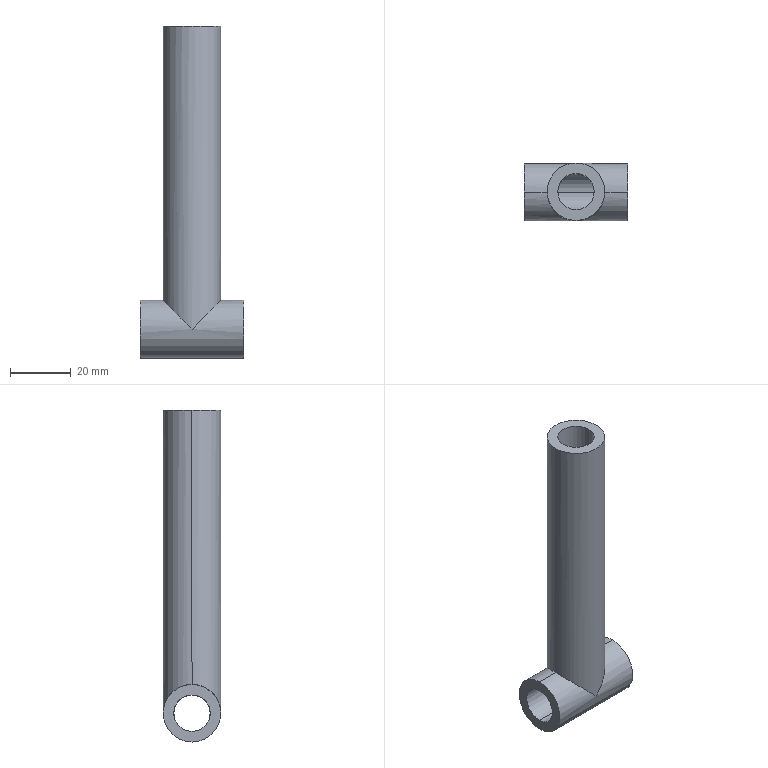Part | NX | features BREP 1 | 1 solid | 11 faces | box 34 x 19 x 109.5 mm | volume 21127 mm3 | cylinder 8 | plane 3 | commonest cylinder face diameters 12 x4 19 x4
STEP:
#1=CARTESIAN_POINT('',(34.,0.,6.));
#2=VERTEX_POINT('',#1);
#3=CARTESIAN_POINT('',(34.,0.,-6.));
#4=VERTEX_POINT('',#3);
#5=CARTESIAN_POINT('',(34.,0.,0.));
#6=DIRECTION('',(1.,0.,0.));
#7=DIRECTION('',(0.,0.,-1.));
#8=AXIS2_PLACEMENT_3D('',#5,#6,#7);
#9=CIRCLE('',#8,6.);
#10=EDGE_CURVE('',#2,#4,#9,.T.);
#11=ORIENTED_EDGE('',*,*,#10,.T.);
#12=CARTESIAN_POINT('',(0.,0.,-6.));
#13=VERTEX_POINT('',#12);
#14=CARTESIAN_POINT('',(34.001,0.,-6.));
#15=DIRECTION('',(-1.,0.,0.));
#16=VECTOR('',#15,1000.);
#17=LINE('',#14,#16);
#18=EDGE_CURVE('',#4,#13,#17,.T.);
#19=ORIENTED_EDGE('',*,*,#18,.T.);
#20=CARTESIAN_POINT('',(0.,0.,6.));
#21=VERTEX_POINT('',#20);
#22=CARTESIAN_POINT('',(0.,0.,0.));
#23=DIRECTION('',(1.,0.,0.));
#24=DIRECTION('',(0.,0.,-1.));
#25=AXIS2_PLACEMENT_3D('',#22,#23,#24);
#26=CIRCLE('',#25,6.);
#27=EDGE_CURVE('',#21,#13,#26,.T.);
#28=ORIENTED_EDGE('',*,*,#27,.F.);
#29=CARTESIAN_POINT('',(11.,0.,6.));
#30=VERTEX_POINT('',#29);
#31=CARTESIAN_POINT('',(34.001,0.,6.));
#32=DIRECTION('',(-1.,0.,0.));
#33=VECTOR('',#32,1000.);
#34=LINE('',#31,#33);
#35=EDGE_CURVE('',#30,#21,#34,.T.);
#36=ORIENTED_EDGE('',*,*,#35,.F.);
#37=CARTESIAN_POINT('',(17.,-6.,0.));
#38=VERTEX_POINT('',#37);
#39=CARTESIAN_POINT('',(11.,0.,6.));
#40=CARTESIAN_POINT('',(11.,-3.515,6.));
#41=CARTESIAN_POINT('',(13.485,-6.,3.515));
#42=CARTESIAN_POINT('',(17.,-6.,0.));
#43=(BOUNDED_CURVE()B_SPLINE_CURVE(3,(#39,#40,#41,#42),.UNSPECIFIED.,.F.,.F.)B_SPLINE_CURVE_WITH_KNOTS((4,4),(0.,1.),.PIECEWISE_BEZIER_KNOTS.)CURVE()GEOMETRIC_REPRESENTATION_ITEM()RATIONAL_B_SPLINE_CURVE((1.,0.8047,0.8047,1.))REPRESENTATION_ITEM(''));
#44=EDGE_CURVE('',#30,#38,#43,.T.);
#45=ORIENTED_EDGE('',*,*,#44,.T.);
#46=CARTESIAN_POINT('',(23.,0.,6.));
#47=VERTEX_POINT('',#46);
#48=CARTESIAN_POINT('',(17.,-6.,0.));
#49=CARTESIAN_POINT('',(20.515,-6.,3.515));
#50=CARTESIAN_POINT('',(23.,-3.515,6.));
#51=CARTESIAN_POINT('',(23.,0.,6.));
#52=(BOUNDED_CURVE()B_SPLINE_CURVE(3,(#48,#49,#50,#51),.UNSPECIFIED.,.F.,.F.)B_SPLINE_CURVE_WITH_KNOTS((4,4),(0.,1.),.PIECEWISE_BEZIER_KNOTS.)CURVE()GEOMETRIC_REPRESENTATION_ITEM()RATIONAL_B_SPLINE_CURVE((1.,0.8047,0.8047,1.))REPRESENTATION_ITEM(''));
#53=EDGE_CURVE('',#38,#47,#52,.T.);
#54=ORIENTED_EDGE('',*,*,#53,.T.);
#55=CARTESIAN_POINT('',(34.001,0.,6.));
#56=DIRECTION('',(-1.,0.,0.));
#57=VECTOR('',#56,1000.);
#58=LINE('',#55,#57);
#59=EDGE_CURVE('',#2,#47,#58,.T.);
#60=ORIENTED_EDGE('',*,*,#59,.F.);
#61=EDGE_LOOP('',(#11,#19,#28,#36,#45,#54,#60));
#62=FACE_BOUND('',#61,.T.);
#63=CARTESIAN_POINT('',(34.001,0.,0.));
#64=DIRECTION('',(-1.,0.,0.));
#65=DIRECTION('',(0.,0.,-1.));
#66=AXIS2_PLACEMENT_3D('',#63,#64,#65);
#67=CYLINDRICAL_SURFACE('',#66,6.);
#68=ADVANCED_FACE('',(#62),#67,.F.);
#69=CARTESIAN_POINT('',(26.5,0.,100.));
#70=VERTEX_POINT('',#69);
#71=CARTESIAN_POINT('',(7.5,0.,100.));
#72=VERTEX_POINT('',#71);
#73=CARTESIAN_POINT('',(17.,0.,100.));
#74=DIRECTION('',(0.,0.,1.));
#75=DIRECTION('',(1.,0.,0.));
#76=AXIS2_PLACEMENT_3D('',#73,#74,#75);
#77=CIRCLE('',#76,9.5);
#78=EDGE_CURVE('',#70,#72,#77,.T.);
#79=ORIENTED_EDGE('',*,*,#78,.F.);
#80=CARTESIAN_POINT('',(26.5,0.,9.5));
#81=VERTEX_POINT('',#80);
#82=CARTESIAN_POINT('',(26.5,0.,100.));
#83=DIRECTION('',(0.,0.,-1.));
#84=VECTOR('',#83,1000.);
#85=LINE('',#82,#84);
#86=EDGE_CURVE('',#81,#70,#85,.F.);
#87=ORIENTED_EDGE('',*,*,#86,.F.);
#88=CARTESIAN_POINT('',(17.,9.5,0.));
#89=VERTEX_POINT('',#88);
#90=CARTESIAN_POINT('',(26.5,0.,9.5));
#91=CARTESIAN_POINT('',(26.5,5.565,9.5));
#92=CARTESIAN_POINT('',(22.565,9.5,5.565));
#93=CARTESIAN_POINT('',(17.,9.5,0.));
#94=(BOUNDED_CURVE()B_SPLINE_CURVE(3,(#90,#91,#92,#93),.UNSPECIFIED.,.F.,.F.)B_SPLINE_CURVE_WITH_KNOTS((4,4),(0.,1.),.PIECEWISE_BEZIER_KNOTS.)CURVE()GEOMETRIC_REPRESENTATION_ITEM()RATIONAL_B_SPLINE_CURVE((1.,0.8047,0.8047,1.))REPRESENTATION_ITEM(''));
#95=EDGE_CURVE('',#81,#89,#94,.T.);
#96=ORIENTED_EDGE('',*,*,#95,.T.);
#97=CARTESIAN_POINT('',(7.5,0.,9.5));
#98=VERTEX_POINT('',#97);
#99=CARTESIAN_POINT('',(17.,9.5,0.));
#100=CARTESIAN_POINT('',(11.435,9.5,5.565));
#101=CARTESIAN_POINT('',(7.5,5.565,9.5));
#102=CARTESIAN_POINT('',(7.5,0.,9.5));
#103=(BOUNDED_CURVE()B_SPLINE_CURVE(3,(#99,#100,#101,#102),.UNSPECIFIED.,.F.,.F.)B_SPLINE_CURVE_WITH_KNOTS((4,4),(0.,1.),.PIECEWISE_BEZIER_KNOTS.)CURVE()GEOMETRIC_REPRESENTATION_ITEM()RATIONAL_B_SPLINE_CURVE((1.,0.8047,0.8047,1.))REPRESENTATION_ITEM(''));
#104=EDGE_CURVE('',#89,#98,#103,.T.);
#105=ORIENTED_EDGE('',*,*,#104,.T.);
#106=CARTESIAN_POINT('',(7.5,0.,100.));
#107=DIRECTION('',(0.,0.,-1.));
#108=VECTOR('',#107,1000.);
#109=LINE('',#106,#108);
#110=EDGE_CURVE('',#98,#72,#109,.F.);
#111=ORIENTED_EDGE('',*,*,#110,.T.);
#112=EDGE_LOOP('',(#79,#87,#96,#105,#111));
#113=FACE_BOUND('',#112,.T.);
#114=CARTESIAN_POINT('',(17.,0.,100.));
#115=DIRECTION('',(0.,0.,-1.));
#116=DIRECTION('',(1.,0.,0.));
#117=AXIS2_PLACEMENT_3D('',#114,#115,#116);
#118=CYLINDRICAL_SURFACE('',#117,9.5);
#119=ADVANCED_FACE('',(#113),#118,.T.);
#120=CARTESIAN_POINT('',(34.,0.,-9.5));
#121=VERTEX_POINT('',#120);
#122=CARTESIAN_POINT('',(34.,0.,9.5));
#123=VERTEX_POINT('',#122);
#124=CARTESIAN_POINT('',(34.,0.,0.));
#125=DIRECTION('',(1.,0.,0.));
#126=DIRECTION('',(0.,0.,-1.));
#127=AXIS2_PLACEMENT_3D('',#124,#125,#126);
#128=CIRCLE('',#127,9.5);
#129=EDGE_CURVE('',#121,#123,#128,.T.);
#130=ORIENTED_EDGE('',*,*,#129,.F.);
#131=CARTESIAN_POINT('',(0.,0.,-9.5));
#132=VERTEX_POINT('',#131);
#133=CARTESIAN_POINT('',(34.,0.,-9.5));
#134=DIRECTION('',(-1.,0.,0.));
#135=VECTOR('',#134,1000.);
#136=LINE('',#133,#135);
#137=EDGE_CURVE('',#121,#132,#136,.T.);
#138=ORIENTED_EDGE('',*,*,#137,.T.);
#139=CARTESIAN_POINT('',(0.,0.,9.5));
#140=VERTEX_POINT('',#139);
#141=CARTESIAN_POINT('',(0.,0.,0.));
#142=DIRECTION('',(1.,0.,0.));
#143=DIRECTION('',(0.,0.,-1.));
#144=AXIS2_PLACEMENT_3D('',#141,#142,#143);
#145=CIRCLE('',#144,9.5);
#146=EDGE_CURVE('',#132,#140,#145,.T.);
#147=ORIENTED_EDGE('',*,*,#146,.T.);
#148=CARTESIAN_POINT('',(34.,0.,9.5));
#149=DIRECTION('',(-1.,0.,0.));
#150=VECTOR('',#149,1000.);
#151=LINE('',#148,#150);
#152=EDGE_CURVE('',#98,#140,#151,.T.);
#153=ORIENTED_EDGE('',*,*,#152,.F.);
#154=ORIENTED_EDGE('',*,*,#104,.F.);
#155=ORIENTED_EDGE('',*,*,#95,.F.);
#156=CARTESIAN_POINT('',(34.,0.,9.5));
#157=DIRECTION('',(-1.,0.,0.));
#158=VECTOR('',#157,1000.);
#159=LINE('',#156,#158);
#160=EDGE_CURVE('',#123,#81,#159,.T.);
#161=ORIENTED_EDGE('',*,*,#160,.F.);
#162=EDGE_LOOP('',(#130,#138,#147,#153,#154,#155,#161));
#163=FACE_BOUND('',#162,.T.);
#164=CARTESIAN_POINT('',(34.,0.,0.));
#165=DIRECTION('',(-1.,0.,0.));
#166=DIRECTION('',(0.,0.,-1.));
#167=AXIS2_PLACEMENT_3D('',#164,#165,#166);
#168=CYLINDRICAL_SURFACE('',#167,9.5);
#169=ADVANCED_FACE('',(#163),#168,.T.);
#170=CARTESIAN_POINT('',(11.,0.,100.));
#171=VERTEX_POINT('',#170);
#172=CARTESIAN_POINT('',(23.,0.,100.));
#173=VERTEX_POINT('',#172);
#174=CARTESIAN_POINT('',(17.,0.,100.));
#175=DIRECTION('',(0.,0.,1.));
#176=DIRECTION('',(1.,0.,0.));
#177=AXIS2_PLACEMENT_3D('',#174,#175,#176);
#178=CIRCLE('',#177,6.);
#179=EDGE_CURVE('',#171,#173,#178,.T.);
#180=ORIENTED_EDGE('',*,*,#179,.T.);
#181=CARTESIAN_POINT('',(23.,0.,100.001));
#182=DIRECTION('',(0.,0.,-1.));
#183=VECTOR('',#182,1000.);
#184=LINE('',#181,#183);
#185=EDGE_CURVE('',#47,#173,#184,.F.);
#186=ORIENTED_EDGE('',*,*,#185,.F.);
#187=ORIENTED_EDGE('',*,*,#53,.F.);
#188=ORIENTED_EDGE('',*,*,#44,.F.);
#189=CARTESIAN_POINT('',(11.,0.,100.001));
#190=DIRECTION('',(0.,0.,-1.));
#191=VECTOR('',#190,1000.);
#192=LINE('',#189,#191);
#193=EDGE_CURVE('',#30,#171,#192,.F.);
#194=ORIENTED_EDGE('',*,*,#193,.T.);
#195=EDGE_LOOP('',(#180,#186,#187,#188,#194));
#196=FACE_BOUND('',#195,.T.);
#197=CARTESIAN_POINT('',(17.,0.,100.001));
#198=DIRECTION('',(0.,0.,-1.));
#199=DIRECTION('',(1.,0.,0.));
#200=AXIS2_PLACEMENT_3D('',#197,#198,#199);
#201=CYLINDRICAL_SURFACE('',#200,6.);
#202=ADVANCED_FACE('',(#196),#201,.F.);
#203=CARTESIAN_POINT('',(34.,0.,0.));
#204=DIRECTION('',(1.,0.,0.));
#205=DIRECTION('',(0.,0.,-1.));
#206=AXIS2_PLACEMENT_3D('',#203,#204,#205);
#207=CIRCLE('',#206,9.5);
#208=EDGE_CURVE('',#123,#121,#207,.T.);
#209=ORIENTED_EDGE('',*,*,#208,.T.);
#210=ORIENTED_EDGE('',*,*,#129,.T.);
#211=EDGE_LOOP('',(#209,#210));
#212=FACE_BOUND('',#211,.T.);
#213=ORIENTED_EDGE('',*,*,#10,.F.);
#214=CARTESIAN_POINT('',(34.,0.,0.));
#215=DIRECTION('',(1.,0.,0.));
#216=DIRECTION('',(0.,0.,-1.));
#217=AXIS2_PLACEMENT_3D('',#214,#215,#216);
#218=CIRCLE('',#217,6.);
#219=EDGE_CURVE('',#4,#2,#218,.T.);
#220=ORIENTED_EDGE('',*,*,#219,.F.);
#221=EDGE_LOOP('',(#213,#220));
#222=FACE_BOUND('',#221,.T.);
#223=CARTESIAN_POINT('',(34.,0.,0.));
#224=DIRECTION('',(1.,0.,0.));
#225=DIRECTION('',(0.,1.,0.));
#226=AXIS2_PLACEMENT_3D('',#223,#224,#225);
#227=PLANE('',#226);
#228=ADVANCED_FACE('',(#212,#222),#227,.T.);
#229=CARTESIAN_POINT('',(0.,0.,0.));
#230=DIRECTION('',(1.,0.,0.));
#231=DIRECTION('',(0.,0.,-1.));
#232=AXIS2_PLACEMENT_3D('',#229,#230,#231);
#233=CIRCLE('',#232,9.5);
#234=EDGE_CURVE('',#140,#132,#233,.T.);
#235=ORIENTED_EDGE('',*,*,#234,.F.);
#236=ORIENTED_EDGE('',*,*,#146,.F.);
#237=EDGE_LOOP('',(#235,#236));
#238=FACE_BOUND('',#237,.T.);
#239=ORIENTED_EDGE('',*,*,#27,.T.);
#240=CARTESIAN_POINT('',(0.,0.,0.));
#241=DIRECTION('',(1.,0.,0.));
#242=DIRECTION('',(0.,0.,-1.));
#243=AXIS2_PLACEMENT_3D('',#240,#241,#242);
#244=CIRCLE('',#243,6.);
#245=EDGE_CURVE('',#13,#21,#244,.T.);
#246=ORIENTED_EDGE('',*,*,#245,.T.);
#247=EDGE_LOOP('',(#239,#246));
#248=FACE_BOUND('',#247,.T.);
#249=CARTESIAN_POINT('',(0.,0.,0.));
#250=DIRECTION('',(1.,0.,0.));
#251=DIRECTION('',(0.,1.,0.));
#252=AXIS2_PLACEMENT_3D('',#249,#250,#251);
#253=PLANE('',#252);
#254=ADVANCED_FACE('',(#238,#248),#253,.F.);
#255=ORIENTED_EDGE('',*,*,#185,.T.);
#256=CARTESIAN_POINT('',(17.,0.,100.));
#257=DIRECTION('',(0.,0.,1.));
#258=DIRECTION('',(1.,0.,0.));
#259=AXIS2_PLACEMENT_3D('',#256,#257,#258);
#260=CIRCLE('',#259,6.);
#261=EDGE_CURVE('',#173,#171,#260,.T.);
#262=ORIENTED_EDGE('',*,*,#261,.T.);
#263=ORIENTED_EDGE('',*,*,#193,.F.);
#264=CARTESIAN_POINT('',(17.,6.,0.));
#265=VERTEX_POINT('',#264);
#266=CARTESIAN_POINT('',(17.,6.,0.));
#267=CARTESIAN_POINT('',(13.485,6.,3.515));
#268=CARTESIAN_POINT('',(11.,3.515,6.));
#269=CARTESIAN_POINT('',(11.,0.,6.));
#270=(BOUNDED_CURVE()B_SPLINE_CURVE(3,(#266,#267,#268,#269),.UNSPECIFIED.,.F.,.F.)B_SPLINE_CURVE_WITH_KNOTS((4,4),(0.,1.),.PIECEWISE_BEZIER_KNOTS.)CURVE()GEOMETRIC_REPRESENTATION_ITEM()RATIONAL_B_SPLINE_CURVE((1.,0.8047,0.8047,1.))REPRESENTATION_ITEM(''));
#271=EDGE_CURVE('',#265,#30,#270,.T.);
#272=ORIENTED_EDGE('',*,*,#271,.F.);
#273=CARTESIAN_POINT('',(23.,0.,6.));
#274=CARTESIAN_POINT('',(23.,3.515,6.));
#275=CARTESIAN_POINT('',(20.515,6.,3.515));
#276=CARTESIAN_POINT('',(17.,6.,0.));
#277=(BOUNDED_CURVE()B_SPLINE_CURVE(3,(#273,#274,#275,#276),.UNSPECIFIED.,.F.,.F.)B_SPLINE_CURVE_WITH_KNOTS((4,4),(0.,1.),.PIECEWISE_BEZIER_KNOTS.)CURVE()GEOMETRIC_REPRESENTATION_ITEM()RATIONAL_B_SPLINE_CURVE((1.,0.8047,0.8047,1.))REPRESENTATION_ITEM(''));
#278=EDGE_CURVE('',#47,#265,#277,.T.);
#279=ORIENTED_EDGE('',*,*,#278,.F.);
#280=EDGE_LOOP('',(#255,#262,#263,#272,#279));
#281=FACE_BOUND('',#280,.T.);
#282=CARTESIAN_POINT('',(17.,0.,100.001));
#283=DIRECTION('',(0.,0.,-1.));
#284=DIRECTION('',(1.,0.,0.));
#285=AXIS2_PLACEMENT_3D('',#282,#283,#284);
#286=CYLINDRICAL_SURFACE('',#285,6.);
#287=ADVANCED_FACE('',(#281),#286,.F.);
#288=CARTESIAN_POINT('',(17.,0.,100.));
#289=DIRECTION('',(0.,0.,1.));
#290=DIRECTION('',(1.,0.,0.));
#291=AXIS2_PLACEMENT_3D('',#288,#289,#290);
#292=CIRCLE('',#291,9.5);
#293=EDGE_CURVE('',#72,#70,#292,.T.);
#294=ORIENTED_EDGE('',*,*,#293,.T.);
#295=ORIENTED_EDGE('',*,*,#78,.T.);
#296=EDGE_LOOP('',(#294,#295));
#297=FACE_BOUND('',#296,.T.);
#298=ORIENTED_EDGE('',*,*,#179,.F.);
#299=ORIENTED_EDGE('',*,*,#261,.F.);
#300=EDGE_LOOP('',(#298,#299));
#301=FACE_BOUND('',#300,.T.);
#302=CARTESIAN_POINT('',(17.,0.,100.));
#303=DIRECTION('',(0.,0.,1.));
#304=DIRECTION('',(-1.,0.,0.));
#305=AXIS2_PLACEMENT_3D('',#302,#303,#304);
#306=PLANE('',#305);
#307=ADVANCED_FACE('',(#297,#301),#306,.T.);
#308=ORIENTED_EDGE('',*,*,#137,.F.);
#309=ORIENTED_EDGE('',*,*,#208,.F.);
#310=ORIENTED_EDGE('',*,*,#160,.T.);
#311=CARTESIAN_POINT('',(17.,-9.5,0.));
#312=VERTEX_POINT('',#311);
#313=CARTESIAN_POINT('',(17.,-9.5,0.));
#314=CARTESIAN_POINT('',(22.565,-9.5,5.565));
#315=CARTESIAN_POINT('',(26.5,-5.565,9.5));
#316=CARTESIAN_POINT('',(26.5,0.,9.5));
#317=(BOUNDED_CURVE()B_SPLINE_CURVE(3,(#313,#314,#315,#316),.UNSPECIFIED.,.F.,.F.)B_SPLINE_CURVE_WITH_KNOTS((4,4),(0.,1.),.PIECEWISE_BEZIER_KNOTS.)CURVE()GEOMETRIC_REPRESENTATION_ITEM()RATIONAL_B_SPLINE_CURVE((1.,0.8047,0.8047,1.))REPRESENTATION_ITEM(''));
#318=EDGE_CURVE('',#312,#81,#317,.T.);
#319=ORIENTED_EDGE('',*,*,#318,.F.);
#320=CARTESIAN_POINT('',(7.5,0.,9.5));
#321=CARTESIAN_POINT('',(7.5,-5.565,9.5));
#322=CARTESIAN_POINT('',(11.435,-9.5,5.565));
#323=CARTESIAN_POINT('',(17.,-9.5,0.));
#324=(BOUNDED_CURVE()B_SPLINE_CURVE(3,(#320,#321,#322,#323),.UNSPECIFIED.,.F.,.F.)B_SPLINE_CURVE_WITH_KNOTS((4,4),(0.,1.),.PIECEWISE_BEZIER_KNOTS.)CURVE()GEOMETRIC_REPRESENTATION_ITEM()RATIONAL_B_SPLINE_CURVE((1.,0.8047,0.8047,1.))REPRESENTATION_ITEM(''));
#325=EDGE_CURVE('',#98,#312,#324,.T.);
#326=ORIENTED_EDGE('',*,*,#325,.F.);
#327=ORIENTED_EDGE('',*,*,#152,.T.);
#328=ORIENTED_EDGE('',*,*,#234,.T.);
#329=EDGE_LOOP('',(#308,#309,#310,#319,#326,#327,#328));
#330=FACE_BOUND('',#329,.T.);
#331=CARTESIAN_POINT('',(34.,0.,0.));
#332=DIRECTION('',(-1.,0.,0.));
#333=DIRECTION('',(0.,0.,-1.));
#334=AXIS2_PLACEMENT_3D('',#331,#332,#333);
#335=CYLINDRICAL_SURFACE('',#334,9.5);
#336=ADVANCED_FACE('',(#330),#335,.T.);
#337=ORIENTED_EDGE('',*,*,#86,.T.);
#338=ORIENTED_EDGE('',*,*,#293,.F.);
#339=ORIENTED_EDGE('',*,*,#110,.F.);
#340=ORIENTED_EDGE('',*,*,#325,.T.);
#341=ORIENTED_EDGE('',*,*,#318,.T.);
#342=EDGE_LOOP('',(#337,#338,#339,#340,#341));
#343=FACE_BOUND('',#342,.T.);
#344=CARTESIAN_POINT('',(17.,0.,100.));
#345=DIRECTION('',(0.,0.,-1.));
#346=DIRECTION('',(1.,0.,0.));
#347=AXIS2_PLACEMENT_3D('',#344,#345,#346);
#348=CYLINDRICAL_SURFACE('',#347,9.5);
#349=ADVANCED_FACE('',(#343),#348,.T.);
#350=ORIENTED_EDGE('',*,*,#18,.F.);
#351=ORIENTED_EDGE('',*,*,#219,.T.);
#352=ORIENTED_EDGE('',*,*,#59,.T.);
#353=ORIENTED_EDGE('',*,*,#278,.T.);
#354=ORIENTED_EDGE('',*,*,#271,.T.);
#355=ORIENTED_EDGE('',*,*,#35,.T.);
#356=ORIENTED_EDGE('',*,*,#245,.F.);
#357=EDGE_LOOP('',(#350,#351,#352,#353,#354,#355,#356));
#358=FACE_BOUND('',#357,.T.);
#359=CARTESIAN_POINT('',(34.001,0.,0.));
#360=DIRECTION('',(-1.,0.,0.));
#361=DIRECTION('',(0.,0.,-1.));
#362=AXIS2_PLACEMENT_3D('',#359,#360,#361);
#363=CYLINDRICAL_SURFACE('',#362,6.);
#364=ADVANCED_FACE('',(#358),#363,.F.);
#365=CLOSED_SHELL('',(#68,#119,#169,#202,#228,#254,#287,#307,#336,#349,#364));
#366=MANIFOLD_SOLID_BREP('',#365);
#367=(LENGTH_UNIT()NAMED_UNIT(*)SI_UNIT(.MILLI.,.METRE.));
#368=UNCERTAINTY_MEASURE_WITH_UNIT(LENGTH_MEASURE(0.00001),#367,'','');
#369=(NAMED_UNIT(*)PLANE_ANGLE_UNIT()SI_UNIT($,.RADIAN.));
#370=(NAMED_UNIT(*)SI_UNIT($,.STERADIAN.)SOLID_ANGLE_UNIT());
#371=(GEOMETRIC_REPRESENTATION_CONTEXT(3)GLOBAL_UNCERTAINTY_ASSIGNED_CONTEXT((#368))GLOBAL_UNIT_ASSIGNED_CONTEXT((#367,#369,#370))REPRESENTATION_CONTEXT('',''));
#372=ADVANCED_BREP_SHAPE_REPRESENTATION('',(#366),#371);